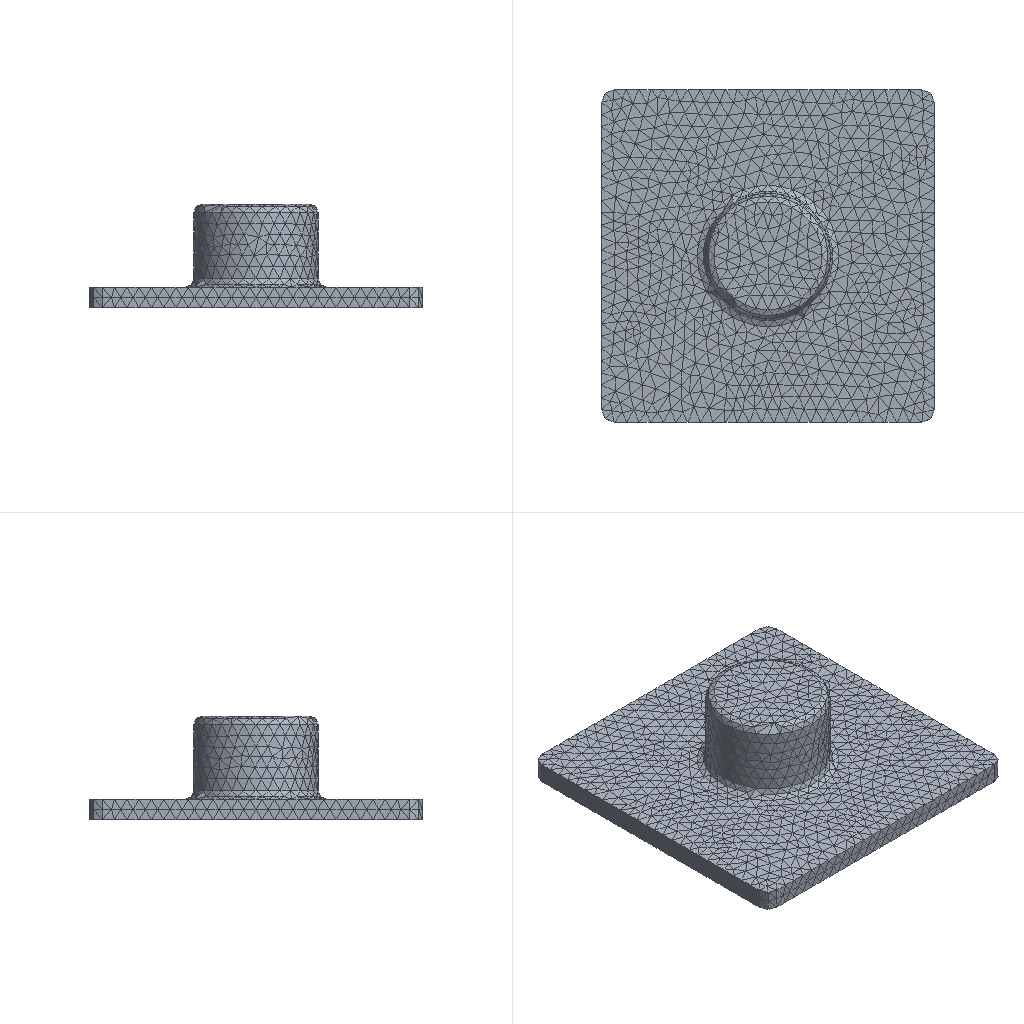Simulation study | ansys workbench
Ansys APDL input file, long lists of numbers shortened:
/batch
/config,noeldb,1     ! force off writing results to database
*get,_wallstrt,active,,time,wall
! ANSYS input file written by Workbench version 2024 R2
! File used for geometry attach:
/title,wbnew--___ (A5)
! ****** Begin Custom Load Command Snippet ******
/COM, ACT Extensions:
/COM,     LSDYNA, 2024.2
/COM,/COM,     ANSYSMotion, 2024.2
/COM,
! ****** End   Custom Load Command Snippet ******
*DIM,_wb_ProjectScratch_dir,string,248
_wb_ProjectScratch_dir(1) = ''
*DIM,_wb_SolverFiles_dir,string,248
_wb_SolverFiles_dir(1) = ''
*DIM,_wb_userfiles_dir,string,248
_wb_userfiles_dir(1) = ''
/com,--- Data in consistent NMM units. See Solving Units in the help system for more information.
/units,MPA
/nopr
/wb,file,start              !  signify a WB generated input file
/prep7
! Turn off shape checking because checks already performed inside WB mesher.
! See help system for more information.
SHPP,OFF,,NOWARN
/nolist
etcon,set             ! allow ANSYS to choose best KEYOP's for 180x elements, resets any applicable keyopt to MAPDL defaults
/com,*********** Nodes for the whole assembly ***********
nblock,3,,26937
(1i9,3e20.9e3)
        1     2.555492712E+03     4.188182850E+03     2.300000000E+01
! (24488 more lines like these left out)
-1
/wb,elem,start            !  set before creation of elements
/com,*********** Elements for Body 1 'Part 1' ***********
et,1,291
eblock,19,solid,,15247
(19i9)
        1        1        1        1        0        0        0        0       10        0        1     2372     3619     2402     3612    19388    19523    19383    19387
! (30493 more lines like these left out)
-1
/wb,elem,end               !  done creating elements
/com,*********** Send User Defined Coordinate System(s) ***********
csys,0
toffst,273.15,      ! Temperature offset from absolute zero
/wb,mat,start              !  starting to send materials
/com,*********** Send Materials ***********
Temperature = 'TEMP' ! Temperature
MP,DENS,1,7.85e-09,	! tonne mm^-3
MP,ALPX,1,1.2e-05,	! C^-1
MP,C,1,434000000,	! mm^2 s^-2 C^-1
MP,KXX,1,60.5,	! tonne mm s^-3 C^-1
MP,RSVX,1,0.00017,	! ohm mm
MP,EX,1,200000,	! tonne s^-2 mm^-1
MP,NUXY,1,0.3,
MP,MURX,1,10000,
/wb,mat,end                !  done sending materials
!************************* Model Summary ********************
!Part 1,	结构钢,	matid,	1
!************************* End Model Summary ********************
! get the diagonal of the bounding box. Needed later for other things
*get,_xmin,node,,mnloc,x
*get,_ymin,node,,mnloc,y
*get,_zmin,node,,mnloc,z
*get,_xmax,node,,mxloc,x
*get,_ymax,node,,mxloc,y
*get,_zmax,node,,mxloc,z
_ASMDIAG=(_xmax-_xmin)*(_xmax-_xmin)+(_ymax-_ymin)*(_ymax-_ymin)+(_zmax-_zmin)*(_zmax-_zmin)
_ASMDIAG=SQRT(_ASMDIAG)
/wb,contact,start          !  starting to send contact
/wb,contact,end            !  done creating contacts
/golist
/wb,load,start             !  starting to send loads
/com,*********** Define Temperature Constraint ***********
CMBLOCK,_CM32   ,NODE,      281
(8i10)
        33        34        35        36        37        38        39        40
! (35 more lines like these left out)
/com,*********** Define Temperature Constraint ***********
CMBLOCK,_CM34   ,NODE,     3125
(8i10)
       237       238       239       242       243       244       245       246
! (390 more lines like these left out)
/com,*********** Define Temperature Constraint ***********
CMBLOCK,_CM45   ,NODE,      840
(8i10)
         1         2         3         4         5         6         7         8
! (104 more lines like these left out)
fcum,add                   ! add nodal forces up (needed in case have loads on the same edge,vertex)
fcum                       ! reset default on fcum command since done sending WB F loads
/com,*********** Create "______" ***********
et,2,152
eblock,10,,,4002
(15i9)
    19250        2        2        2        0      244      245     1928     1928     5448     5457     1928     5452
! (4001 more lines like these left out)
-1
esel,s,type,,2
keyop,2,8,5
keyop,2,13,0
*DIM,_convvari47,TABLE,8,1,1,TEMP, , ,0
! Temperature values
*TAXIS,_convvari47(1),1,1.,10.,100.,200.,300.,500.,700.,1000.
! Load values
_convvari47(1,1,1) = 1.24e-003
_convvari47(2,1,1) = 2.67e-003
_convvari47(3,1,1) = 5.76e-003
_convvari47(4,1,1) = 7.25e-003
_convvari47(5,1,1) = 8.3e-003
_convvari47(6,1,1) = 9.84e-003
_convvari47(7,1,1) = 1.101e-002
_convvari47(8,1,1) = 1.24e-002
esel,all
/com,***************** Define Uniform Initial temperature ***************
tunif,22.
/gst,on,on
fini
*get,_numnode,node,0,count
*get,_numelem,elem,0,count
*get, _MAXELEMNUM, elem, 0, NUM, MAX
*get, _MAXNODENUM, node, 0, NUM, MAX
*get, _MAXELEMTYPE, etyp, 0, NUM, MAX
*get, _MAXREALCONST, rcon, 0, NUM, MAX
/go
/wb,load,end               !  done creating loads
/com,--- Number of total nodes = %_numnode%
/com,--- Number of contact elements = 4002
/com,--- Number of spring elements = 0
/com,--- Number of bearing elements = 0
/com,--- Number of solid elements = 15247
/com,--- Number of condensed parts = 0
/com,--- Number of total elements = %_numelem%
*get,_wallbsol,active,,time,wall
/com,****************************************************************************
/com,*************************    SOLUTION       ********************************
/com,****************************************************************************
/solu
antype,0                   ! static analysis
!eqsl,sparse               ! using sparse solver which is default so no eqsl command needed
cntr,print,1               ! print out contact info and also make no initial contact an error
cncheck,dmp		!	Enable program controlled contact splitting for distributed memory parallel run
rescontrol,,none                 ! Do not keep any restart files
dmpoption,emat,no             ! Don't combine emat file for DANSYS
dmpoption,esav,no             ! Don't combine esav file for DANSYS
/com,****************************************************
/com,******************* SOLVE FOR LS 1 OF 1 ****************
d,_CM32,temp,150.
d,_CM34,temp,30.
d,_CM45,temp,80.
esel,s,type,,2
nsle
sf,all,conv,%_convvari47%,22.
nsel,all
esel,all
/nopr
/gopr
autots,on
nsub,1,10,1
time,1.
outres,erase
outres,all,none
outres,nsol,all
outres,rsol,all
outres,eangl,all
outres,veng,all
outres,fflux,all,
outres,cont,all,
/nopr
esel,s,type,,2
cm,_elmisc,elem
esel,all
/gopr
outres,misc,all,_elmisc
cnvtol,heat,,1.e-003,,1.e-003 ! Program Controlled. Set MINREF equivalent of 1e-6 Watts
! *********** WB SOLVE COMMAND ***********
! check interactive state
*get,ANSINTER_,active,,int
*if,ANSINTER_,ne,0,then
/eof
*endif
solve
/com *************** Write FE CONNECTORS *********
CEWRITE,file,ce,,INTE
/com,****************************************************
/com,*************** FINISHED SOLVE FOR LS 1 *************
*get,_wallasol,active,,time,wall
/post1
xmlo,ENCODING,ISO-8859-1
xmlo,parm
/xml,parm,xml
fini
/gopr
*get,_walldone,active,,time,wall
_preptime=(_wallbsol-_wallstrt)*3600
_solvtime=(_wallasol-_wallbsol)*3600
_posttime=(_walldone-_wallasol)*3600
_totaltim=(_walldone-_wallstrt)*3600
*get,_dlbratio,active,0,solu,dlbr
*get,_combtime,active,0,solu,comb
*get,_ssmode,active,0,solu,ssmm
*get,_ndofs,active,0,solu,ndof
/fclean				!clean distributed files
/com,--- Total number of nodes = %_numnode%
/com,--- Total number of elements = %_numelem%
/com,--- Element load balance ratio = %_dlbratio%
/com,--- Time to combine distributed files = %_combtime%
/com,--- Sparse memory mode = %_ssmode%
/com,--- Number of DOF = %_ndofs%
/wb,file,end               ! done with WB generated input